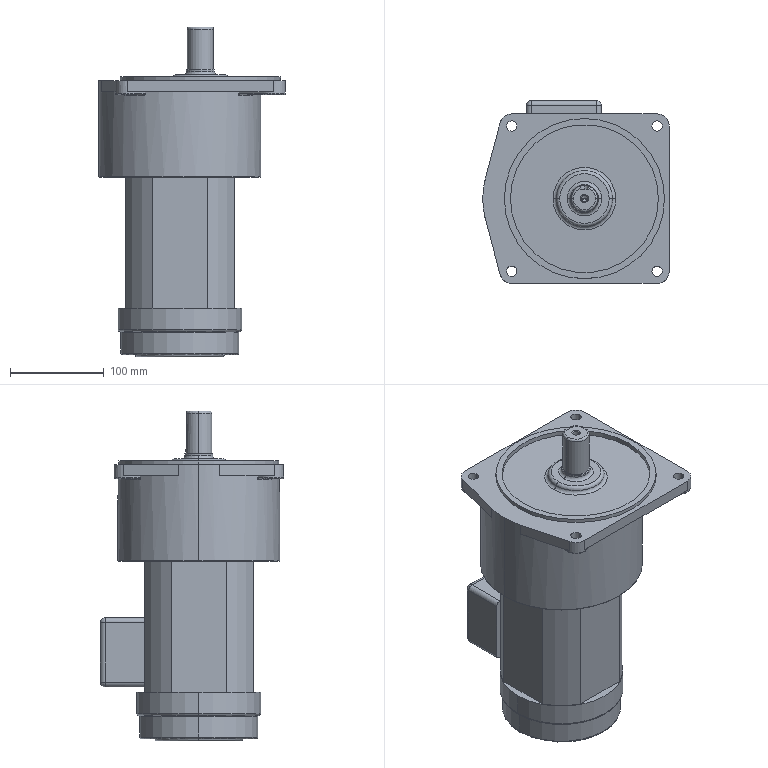Part | STEP file | 102000010058 | 1 solid | 170 faces | box 199 x 195.5 x 352 mm | volume 5244332 mm3 | cylinder 66 | plane 47 | torus 41 | spline 8 | cone 4 | sphere 4 | commonest cylinder face diameters 2 x20 10 x8 11 x8 26 x8 130 x4 6.8 x2